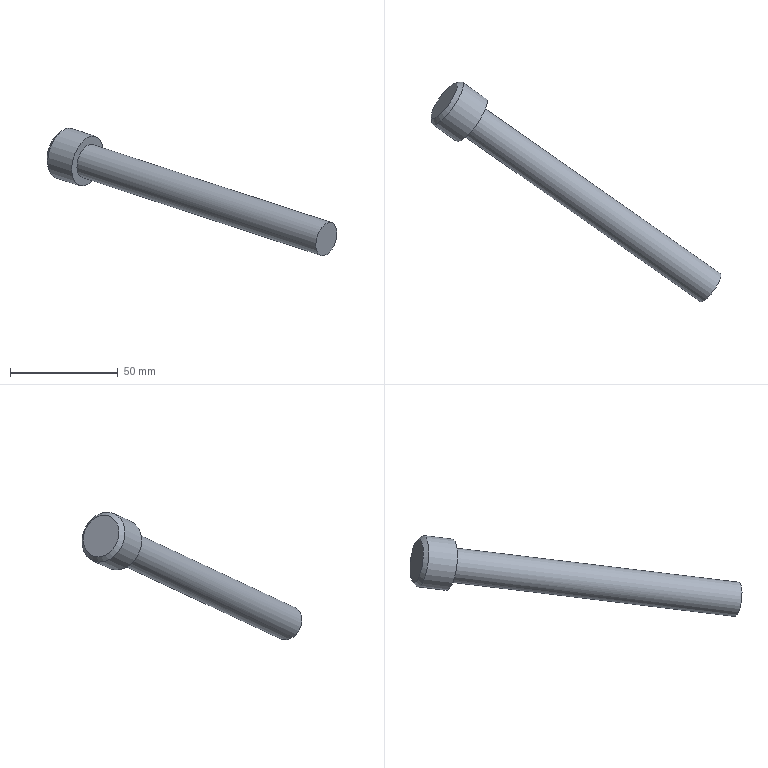Part | NX | features solid 2 | 1 solid | 6 faces | box 134.441 x 101.971 x 59.177 mm | volume 35244 mm3 | plane 3 | cylinder 2 | cone 1 | commonest cylinder face diameters 16 x1 24 x1
STEP:
#1=CARTESIAN_POINT('',(-218.179,754.113,30.414));
#2=VERTEX_POINT('',#1);
#3=CARTESIAN_POINT('',(-220.736,747.271,37.244));
#4=DIRECTION('',(0.7912,-0.554,-0.2588));
#5=DIRECTION('',(0.2557,0.6842,-0.683));
#6=AXIS2_PLACEMENT_3D('',#3,#4,#5);
#7=CIRCLE('',#6,10.);
#8=EDGE_CURVE('',#2,#2,#7,.T.);
#9=ORIENTED_EDGE('',*,*,#8,.F.);
#10=EDGE_LOOP('',(#9));
#11=FACE_BOUND('',#10,.T.);
#12=CARTESIAN_POINT('',(-220.736,747.271,37.244));
#13=DIRECTION('',(-0.7912,0.554,0.2588));
#14=DIRECTION('',(0.2557,0.6842,-0.683));
#15=AXIS2_PLACEMENT_3D('',#12,#13,#14);
#16=PLANE('',#15);
#17=ADVANCED_FACE('',(#11),#16,.T.);
#18=CARTESIAN_POINT('',(-210.121,732.933,38.567));
#19=VERTEX_POINT('',#18);
#20=CARTESIAN_POINT('',(-208.076,738.407,33.103));
#21=DIRECTION('',(-0.7912,0.554,0.2588));
#22=DIRECTION('',(-0.2557,-0.6842,0.683));
#23=AXIS2_PLACEMENT_3D('',#20,#21,#22);
#24=CIRCLE('',#23,8.);
#25=EDGE_CURVE('',#19,#19,#24,.T.);
#26=ORIENTED_EDGE('',*,*,#25,.T.);
#27=EDGE_LOOP('',(#26));
#28=FACE_BOUND('',#27,.T.);
#29=CARTESIAN_POINT('',(-205.008,746.617,24.907));
#30=VERTEX_POINT('',#29);
#31=CARTESIAN_POINT('',(-208.076,738.407,33.103));
#32=DIRECTION('',(0.7912,-0.554,-0.2588));
#33=DIRECTION('',(0.2557,0.6842,-0.683));
#34=AXIS2_PLACEMENT_3D('',#31,#32,#33);
#35=CIRCLE('',#34,12.);
#36=EDGE_CURVE('',#30,#30,#35,.T.);
#37=ORIENTED_EDGE('',*,*,#36,.T.);
#38=EDGE_LOOP('',(#37));
#39=FACE_BOUND('',#38,.T.);
#40=CARTESIAN_POINT('',(-208.076,738.407,33.103));
#41=DIRECTION('',(0.7912,-0.554,-0.2588));
#42=DIRECTION('',(-0.2557,-0.6842,0.683));
#43=AXIS2_PLACEMENT_3D('',#40,#41,#42);
#44=PLANE('',#43);
#45=ADVANCED_FACE('',(#28,#39),#44,.T.);
#46=CARTESIAN_POINT('',(-216.086,754.373,28.53));
#47=VERTEX_POINT('',#46);
#48=CARTESIAN_POINT('',(-219.153,746.163,36.727));
#49=DIRECTION('',(0.7912,-0.554,-0.2588));
#50=DIRECTION('',(0.2557,0.6842,-0.683));
#51=AXIS2_PLACEMENT_3D('',#48,#49,#50);
#52=CIRCLE('',#51,12.);
#53=EDGE_CURVE('',#47,#47,#52,.F.);
#54=ORIENTED_EDGE('',*,*,#53,.F.);
#55=EDGE_LOOP('',(#54));
#56=FACE_BOUND('',#55,.T.);
#57=ORIENTED_EDGE('',*,*,#36,.F.);
#58=EDGE_LOOP('',(#57));
#59=FACE_BOUND('',#58,.T.);
#60=CARTESIAN_POINT('',(-208.076,738.407,33.103));
#61=DIRECTION('',(-0.7912,0.554,0.2588));
#62=DIRECTION('',(0.2557,0.6842,-0.683));
#63=AXIS2_PLACEMENT_3D('',#60,#61,#62);
#64=CYLINDRICAL_SURFACE('',#63,12.);
#65=ADVANCED_FACE('',(#56,#59),#64,.T.);
#66=CARTESIAN_POINT('',(-101.891,654.289,-3.132));
#67=VERTEX_POINT('',#66);
#68=CARTESIAN_POINT('',(-97.303,660.842,-3.132));
#69=DIRECTION('',(-0.7912,0.554,0.2588));
#70=DIRECTION('',(-0.5736,-0.8192,0.));
#71=AXIS2_PLACEMENT_3D('',#68,#69,#70);
#72=CIRCLE('',#71,8.);
#73=EDGE_CURVE('',#67,#67,#72,.F.);
#74=ORIENTED_EDGE('',*,*,#73,.T.);
#75=EDGE_LOOP('',(#74));
#76=FACE_BOUND('',#75,.T.);
#77=CARTESIAN_POINT('',(-97.303,660.842,-3.132));
#78=DIRECTION('',(0.7912,-0.554,-0.2588));
#79=DIRECTION('',(-0.2557,-0.6842,0.683));
#80=AXIS2_PLACEMENT_3D('',#77,#78,#79);
#81=PLANE('',#80);
#82=ADVANCED_FACE('',(#76),#81,.T.);
#83=ORIENTED_EDGE('',*,*,#73,.F.);
#84=EDGE_LOOP('',(#83));
#85=FACE_BOUND('',#84,.T.);
#86=ORIENTED_EDGE('',*,*,#25,.F.);
#87=EDGE_LOOP('',(#86));
#88=FACE_BOUND('',#87,.T.);
#89=CARTESIAN_POINT('',(-208.076,738.407,33.103));
#90=DIRECTION('',(0.7912,-0.554,-0.2588));
#91=DIRECTION('',(-0.2557,-0.6842,0.683));
#92=AXIS2_PLACEMENT_3D('',#89,#90,#91);
#93=CYLINDRICAL_SURFACE('',#92,8.);
#94=ADVANCED_FACE('',(#85,#88),#93,.T.);
#95=ORIENTED_EDGE('',*,*,#8,.T.);
#96=EDGE_LOOP('',(#95));
#97=FACE_BOUND('',#96,.T.);
#98=ORIENTED_EDGE('',*,*,#53,.T.);
#99=EDGE_LOOP('',(#98));
#100=FACE_BOUND('',#99,.T.);
#101=CARTESIAN_POINT('',(-219.153,746.163,36.727));
#102=DIRECTION('',(0.7912,-0.554,-0.2588));
#103=DIRECTION('',(-0.2557,-0.6842,0.683));
#104=AXIS2_PLACEMENT_3D('',#101,#102,#103);
#105=CONICAL_SURFACE('',#104,12.,0.7854);
#106=ADVANCED_FACE('',(#97,#100),#105,.T.);
#107=CLOSED_SHELL('',(#17,#45,#65,#82,#94,#106));
#108=MANIFOLD_SOLID_BREP('',#107);
#109=(LENGTH_UNIT()NAMED_UNIT(*)SI_UNIT(.MILLI.,.METRE.));
#110=UNCERTAINTY_MEASURE_WITH_UNIT(LENGTH_MEASURE(0.00001),#109,'','');
#111=(NAMED_UNIT(*)PLANE_ANGLE_UNIT()SI_UNIT($,.RADIAN.));
#112=(NAMED_UNIT(*)SI_UNIT($,.STERADIAN.)SOLID_ANGLE_UNIT());
#113=(GEOMETRIC_REPRESENTATION_CONTEXT(3)GLOBAL_UNCERTAINTY_ASSIGNED_CONTEXT((#110))GLOBAL_UNIT_ASSIGNED_CONTEXT((#109,#111,#112))REPRESENTATION_CONTEXT('',''));
#114=ADVANCED_BREP_SHAPE_REPRESENTATION('',(#108),#113);